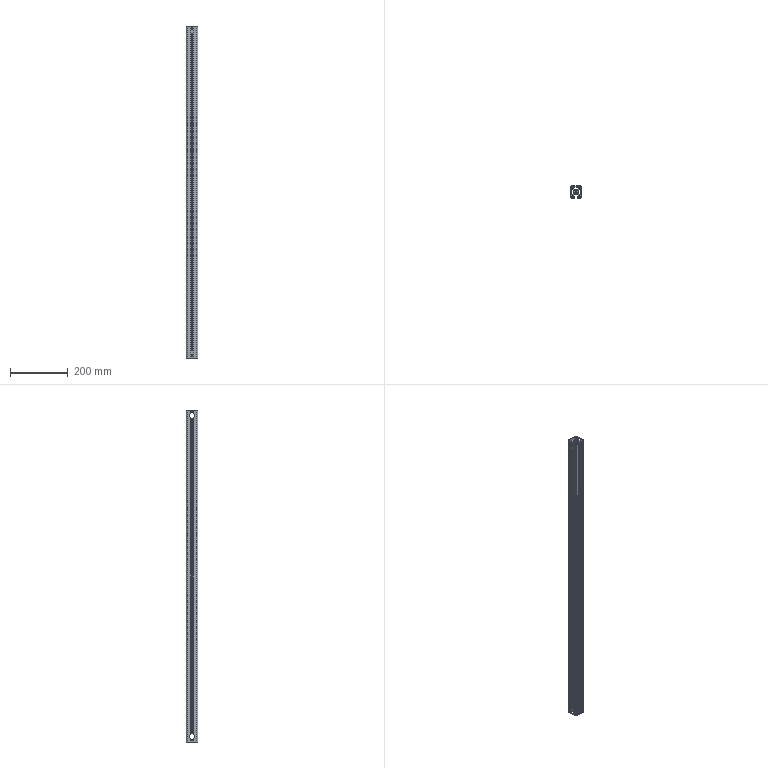Part | SolidWorks | features BaseBody 1, HoleWzd 1, MoveFace 1 | 1 solid | 242 faces | box 40 x 40 x 1146 mm | volume 670131 mm3 | plane 187 | cylinder 55 | commonest cylinder face diameters 6.8 x15 2 x14 19 x12 1 x6 5 x4 9 x4